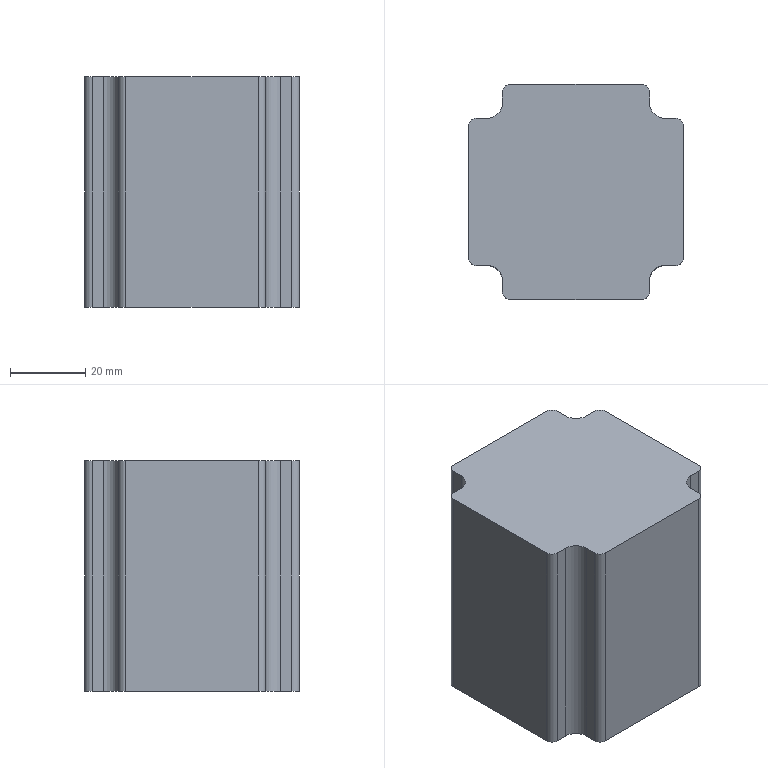Part | SolidWorks | features BaseBody 1 | 1 solid | 26 faces | box 57 x 57 x 61 mm | volume 178844 mm3 | plane 14 | cylinder 12 | commonest cylinder face diameters 4 x8 8 x4
STEP:
#1=CARTESIAN_POINT('',(19.5,26.5,0.));
#2=VERTEX_POINT('',#1);
#3=CARTESIAN_POINT('',(17.5,28.5,0.));
#4=VERTEX_POINT('',#3);
#5=CARTESIAN_POINT('',(17.5,26.5,0.));
#6=DIRECTION('',(0.,0.,1.));
#7=DIRECTION('',(-1.,0.,0.));
#8=AXIS2_PLACEMENT_3D('',#5,#6,#7);
#9=CIRCLE('',#8,2.);
#10=EDGE_CURVE('',#2,#4,#9,.T.);
#11=ORIENTED_EDGE('',*,*,#10,.T.);
#12=CARTESIAN_POINT('',(17.5,28.5,61.));
#13=VERTEX_POINT('',#12);
#14=CARTESIAN_POINT('',(17.5,28.5,61.));
#15=DIRECTION('',(0.,0.,-1.));
#16=VECTOR('',#15,1000.);
#17=LINE('',#14,#16);
#18=EDGE_CURVE('',#13,#4,#17,.T.);
#19=ORIENTED_EDGE('',*,*,#18,.F.);
#20=CARTESIAN_POINT('',(19.5,26.5,61.));
#21=VERTEX_POINT('',#20);
#22=CARTESIAN_POINT('',(17.5,26.5,61.));
#23=DIRECTION('',(0.,0.,1.));
#24=DIRECTION('',(-1.,0.,0.));
#25=AXIS2_PLACEMENT_3D('',#22,#23,#24);
#26=CIRCLE('',#25,2.);
#27=EDGE_CURVE('',#21,#13,#26,.T.);
#28=ORIENTED_EDGE('',*,*,#27,.F.);
#29=CARTESIAN_POINT('',(19.5,26.5,61.));
#30=DIRECTION('',(0.,0.,-1.));
#31=VECTOR('',#30,1000.);
#32=LINE('',#29,#31);
#33=EDGE_CURVE('',#21,#2,#32,.T.);
#34=ORIENTED_EDGE('',*,*,#33,.T.);
#35=EDGE_LOOP('',(#11,#19,#28,#34));
#36=FACE_OUTER_BOUND('',#35,.T.);
#37=CARTESIAN_POINT('',(17.5,26.5,61.));
#38=DIRECTION('',(0.,0.,-1.));
#39=DIRECTION('',(-1.,0.,0.));
#40=AXIS2_PLACEMENT_3D('',#37,#38,#39);
#41=CYLINDRICAL_SURFACE('',#40,2.);
#42=ADVANCED_FACE('',(#36),#41,.T.);
#43=CARTESIAN_POINT('',(-17.5,28.5,0.));
#44=VERTEX_POINT('',#43);
#45=CARTESIAN_POINT('',(-17.5,28.5,0.));
#46=DIRECTION('',(-1.,0.,0.));
#47=VECTOR('',#46,1000.);
#48=LINE('',#45,#47);
#49=EDGE_CURVE('',#4,#44,#48,.T.);
#50=ORIENTED_EDGE('',*,*,#49,.T.);
#51=CARTESIAN_POINT('',(-17.5,28.5,61.));
#52=VERTEX_POINT('',#51);
#53=CARTESIAN_POINT('',(-17.5,28.5,61.));
#54=DIRECTION('',(0.,0.,-1.));
#55=VECTOR('',#54,1000.);
#56=LINE('',#53,#55);
#57=EDGE_CURVE('',#52,#44,#56,.T.);
#58=ORIENTED_EDGE('',*,*,#57,.F.);
#59=CARTESIAN_POINT('',(-17.5,28.5,61.));
#60=DIRECTION('',(-1.,0.,0.));
#61=VECTOR('',#60,1000.);
#62=LINE('',#59,#61);
#63=EDGE_CURVE('',#13,#52,#62,.T.);
#64=ORIENTED_EDGE('',*,*,#63,.F.);
#65=ORIENTED_EDGE('',*,*,#18,.T.);
#66=EDGE_LOOP('',(#50,#58,#64,#65));
#67=FACE_OUTER_BOUND('',#66,.T.);
#68=CARTESIAN_POINT('',(-17.5,28.5,61.));
#69=DIRECTION('',(0.,-1.,0.));
#70=DIRECTION('',(0.,0.,-1.));
#71=AXIS2_PLACEMENT_3D('',#68,#69,#70);
#72=PLANE('',#71);
#73=ADVANCED_FACE('',(#67),#72,.F.);
#74=CARTESIAN_POINT('',(-19.5,26.5,0.));
#75=VERTEX_POINT('',#74);
#76=CARTESIAN_POINT('',(-17.5,26.5,0.));
#77=DIRECTION('',(0.,0.,1.));
#78=DIRECTION('',(-1.,0.,0.));
#79=AXIS2_PLACEMENT_3D('',#76,#77,#78);
#80=CIRCLE('',#79,2.);
#81=EDGE_CURVE('',#44,#75,#80,.T.);
#82=ORIENTED_EDGE('',*,*,#81,.T.);
#83=CARTESIAN_POINT('',(-19.5,26.5,61.));
#84=VERTEX_POINT('',#83);
#85=CARTESIAN_POINT('',(-19.5,26.5,61.));
#86=DIRECTION('',(0.,0.,-1.));
#87=VECTOR('',#86,1000.);
#88=LINE('',#85,#87);
#89=EDGE_CURVE('',#84,#75,#88,.T.);
#90=ORIENTED_EDGE('',*,*,#89,.F.);
#91=CARTESIAN_POINT('',(-17.5,26.5,61.));
#92=DIRECTION('',(0.,0.,1.));
#93=DIRECTION('',(-1.,0.,0.));
#94=AXIS2_PLACEMENT_3D('',#91,#92,#93);
#95=CIRCLE('',#94,2.);
#96=EDGE_CURVE('',#52,#84,#95,.T.);
#97=ORIENTED_EDGE('',*,*,#96,.F.);
#98=ORIENTED_EDGE('',*,*,#57,.T.);
#99=EDGE_LOOP('',(#82,#90,#97,#98));
#100=FACE_OUTER_BOUND('',#99,.T.);
#101=CARTESIAN_POINT('',(-17.5,26.5,61.));
#102=DIRECTION('',(0.,0.,-1.));
#103=DIRECTION('',(-1.,0.,0.));
#104=AXIS2_PLACEMENT_3D('',#101,#102,#103);
#105=CYLINDRICAL_SURFACE('',#104,2.);
#106=ADVANCED_FACE('',(#100),#105,.T.);
#107=CARTESIAN_POINT('',(-19.5,23.5,0.));
#108=VERTEX_POINT('',#107);
#109=CARTESIAN_POINT('',(-19.5,23.5,0.));
#110=DIRECTION('',(0.,-1.,0.));
#111=VECTOR('',#110,1000.);
#112=LINE('',#109,#111);
#113=EDGE_CURVE('',#75,#108,#112,.T.);
#114=ORIENTED_EDGE('',*,*,#113,.T.);
#115=CARTESIAN_POINT('',(-19.5,23.5,61.));
#116=VERTEX_POINT('',#115);
#117=CARTESIAN_POINT('',(-19.5,23.5,61.));
#118=DIRECTION('',(0.,0.,-1.));
#119=VECTOR('',#118,1000.);
#120=LINE('',#117,#119);
#121=EDGE_CURVE('',#116,#108,#120,.T.);
#122=ORIENTED_EDGE('',*,*,#121,.F.);
#123=CARTESIAN_POINT('',(-19.5,23.5,61.));
#124=DIRECTION('',(0.,-1.,0.));
#125=VECTOR('',#124,1000.);
#126=LINE('',#123,#125);
#127=EDGE_CURVE('',#84,#116,#126,.T.);
#128=ORIENTED_EDGE('',*,*,#127,.F.);
#129=ORIENTED_EDGE('',*,*,#89,.T.);
#130=EDGE_LOOP('',(#114,#122,#128,#129));
#131=FACE_OUTER_BOUND('',#130,.T.);
#132=CARTESIAN_POINT('',(-19.5,23.5,61.));
#133=DIRECTION('',(1.,0.,0.));
#134=DIRECTION('',(0.,1.,0.));
#135=AXIS2_PLACEMENT_3D('',#132,#133,#134);
#136=PLANE('',#135);
#137=ADVANCED_FACE('',(#131),#136,.F.);
#138=CARTESIAN_POINT('',(-23.5,19.5,0.));
#139=VERTEX_POINT('',#138);
#140=CARTESIAN_POINT('',(-23.5,23.5,0.));
#141=DIRECTION('',(0.,0.,-1.));
#142=DIRECTION('',(1.,0.,0.));
#143=AXIS2_PLACEMENT_3D('',#140,#141,#142);
#144=CIRCLE('',#143,4.);
#145=EDGE_CURVE('',#108,#139,#144,.T.);
#146=ORIENTED_EDGE('',*,*,#145,.T.);
#147=CARTESIAN_POINT('',(-23.5,19.5,61.));
#148=VERTEX_POINT('',#147);
#149=CARTESIAN_POINT('',(-23.5,19.5,61.));
#150=DIRECTION('',(0.,0.,-1.));
#151=VECTOR('',#150,1000.);
#152=LINE('',#149,#151);
#153=EDGE_CURVE('',#148,#139,#152,.T.);
#154=ORIENTED_EDGE('',*,*,#153,.F.);
#155=CARTESIAN_POINT('',(-23.5,23.5,61.));
#156=DIRECTION('',(0.,0.,-1.));
#157=DIRECTION('',(1.,0.,0.));
#158=AXIS2_PLACEMENT_3D('',#155,#156,#157);
#159=CIRCLE('',#158,4.);
#160=EDGE_CURVE('',#116,#148,#159,.T.);
#161=ORIENTED_EDGE('',*,*,#160,.F.);
#162=ORIENTED_EDGE('',*,*,#121,.T.);
#163=EDGE_LOOP('',(#146,#154,#161,#162));
#164=FACE_OUTER_BOUND('',#163,.T.);
#165=CARTESIAN_POINT('',(-23.5,23.5,61.));
#166=DIRECTION('',(0.,0.,-1.));
#167=DIRECTION('',(-1.,0.,0.));
#168=AXIS2_PLACEMENT_3D('',#165,#166,#167);
#169=CYLINDRICAL_SURFACE('',#168,4.);
#170=ADVANCED_FACE('',(#164),#169,.F.);
#171=CARTESIAN_POINT('',(-26.5,19.5,0.));
#172=VERTEX_POINT('',#171);
#173=CARTESIAN_POINT('',(-26.5,19.5,0.));
#174=DIRECTION('',(-1.,0.,0.));
#175=VECTOR('',#174,1000.);
#176=LINE('',#173,#175);
#177=EDGE_CURVE('',#139,#172,#176,.T.);
#178=ORIENTED_EDGE('',*,*,#177,.T.);
#179=CARTESIAN_POINT('',(-26.5,19.5,61.));
#180=VERTEX_POINT('',#179);
#181=CARTESIAN_POINT('',(-26.5,19.5,61.));
#182=DIRECTION('',(0.,0.,-1.));
#183=VECTOR('',#182,1000.);
#184=LINE('',#181,#183);
#185=EDGE_CURVE('',#180,#172,#184,.T.);
#186=ORIENTED_EDGE('',*,*,#185,.F.);
#187=CARTESIAN_POINT('',(-26.5,19.5,61.));
#188=DIRECTION('',(-1.,0.,0.));
#189=VECTOR('',#188,1000.);
#190=LINE('',#187,#189);
#191=EDGE_CURVE('',#148,#180,#190,.T.);
#192=ORIENTED_EDGE('',*,*,#191,.F.);
#193=ORIENTED_EDGE('',*,*,#153,.T.);
#194=EDGE_LOOP('',(#178,#186,#192,#193));
#195=FACE_OUTER_BOUND('',#194,.T.);
#196=CARTESIAN_POINT('',(-26.5,19.5,61.));
#197=DIRECTION('',(0.,-1.,0.));
#198=DIRECTION('',(0.,0.,-1.));
#199=AXIS2_PLACEMENT_3D('',#196,#197,#198);
#200=PLANE('',#199);
#201=ADVANCED_FACE('',(#195),#200,.F.);
#202=CARTESIAN_POINT('',(-28.5,17.5,0.));
#203=VERTEX_POINT('',#202);
#204=CARTESIAN_POINT('',(-26.5,17.5,0.));
#205=DIRECTION('',(0.,0.,1.));
#206=DIRECTION('',(-1.,0.,0.));
#207=AXIS2_PLACEMENT_3D('',#204,#205,#206);
#208=CIRCLE('',#207,2.);
#209=EDGE_CURVE('',#172,#203,#208,.T.);
#210=ORIENTED_EDGE('',*,*,#209,.T.);
#211=CARTESIAN_POINT('',(-28.5,17.5,61.));
#212=VERTEX_POINT('',#211);
#213=CARTESIAN_POINT('',(-28.5,17.5,61.));
#214=DIRECTION('',(0.,0.,-1.));
#215=VECTOR('',#214,1000.);
#216=LINE('',#213,#215);
#217=EDGE_CURVE('',#212,#203,#216,.T.);
#218=ORIENTED_EDGE('',*,*,#217,.F.);
#219=CARTESIAN_POINT('',(-26.5,17.5,61.));
#220=DIRECTION('',(0.,0.,1.));
#221=DIRECTION('',(-1.,0.,0.));
#222=AXIS2_PLACEMENT_3D('',#219,#220,#221);
#223=CIRCLE('',#222,2.);
#224=EDGE_CURVE('',#180,#212,#223,.T.);
#225=ORIENTED_EDGE('',*,*,#224,.F.);
#226=ORIENTED_EDGE('',*,*,#185,.T.);
#227=EDGE_LOOP('',(#210,#218,#225,#226));
#228=FACE_OUTER_BOUND('',#227,.T.);
#229=CARTESIAN_POINT('',(-26.5,17.5,61.));
#230=DIRECTION('',(0.,0.,-1.));
#231=DIRECTION('',(-1.,0.,0.));
#232=AXIS2_PLACEMENT_3D('',#229,#230,#231);
#233=CYLINDRICAL_SURFACE('',#232,2.);
#234=ADVANCED_FACE('',(#228),#233,.T.);
#235=CARTESIAN_POINT('',(-28.5,-17.5,0.));
#236=VERTEX_POINT('',#235);
#237=CARTESIAN_POINT('',(-28.5,-17.5,0.));
#238=DIRECTION('',(0.,-1.,0.));
#239=VECTOR('',#238,1000.);
#240=LINE('',#237,#239);
#241=EDGE_CURVE('',#203,#236,#240,.T.);
#242=ORIENTED_EDGE('',*,*,#241,.T.);
#243=CARTESIAN_POINT('',(-28.5,-17.5,61.));
#244=VERTEX_POINT('',#243);
#245=CARTESIAN_POINT('',(-28.5,-17.5,61.));
#246=DIRECTION('',(0.,0.,-1.));
#247=VECTOR('',#246,1000.);
#248=LINE('',#245,#247);
#249=EDGE_CURVE('',#244,#236,#248,.T.);
#250=ORIENTED_EDGE('',*,*,#249,.F.);
#251=CARTESIAN_POINT('',(-28.5,-17.5,61.));
#252=DIRECTION('',(0.,-1.,0.));
#253=VECTOR('',#252,1000.);
#254=LINE('',#251,#253);
#255=EDGE_CURVE('',#212,#244,#254,.T.);
#256=ORIENTED_EDGE('',*,*,#255,.F.);
#257=ORIENTED_EDGE('',*,*,#217,.T.);
#258=EDGE_LOOP('',(#242,#250,#256,#257));
#259=FACE_OUTER_BOUND('',#258,.T.);
#260=CARTESIAN_POINT('',(-28.5,-17.5,61.));
#261=DIRECTION('',(1.,0.,0.));
#262=DIRECTION('',(0.,1.,0.));
#263=AXIS2_PLACEMENT_3D('',#260,#261,#262);
#264=PLANE('',#263);
#265=ADVANCED_FACE('',(#259),#264,.F.);
#266=CARTESIAN_POINT('',(-26.5,-19.5,0.));
#267=VERTEX_POINT('',#266);
#268=CARTESIAN_POINT('',(-26.5,-17.5,0.));
#269=DIRECTION('',(0.,0.,1.));
#270=DIRECTION('',(-1.,0.,0.));
#271=AXIS2_PLACEMENT_3D('',#268,#269,#270);
#272=CIRCLE('',#271,2.);
#273=EDGE_CURVE('',#236,#267,#272,.T.);
#274=ORIENTED_EDGE('',*,*,#273,.T.);
#275=CARTESIAN_POINT('',(-26.5,-19.5,61.));
#276=VERTEX_POINT('',#275);
#277=CARTESIAN_POINT('',(-26.5,-19.5,61.));
#278=DIRECTION('',(0.,0.,-1.));
#279=VECTOR('',#278,1000.);
#280=LINE('',#277,#279);
#281=EDGE_CURVE('',#276,#267,#280,.T.);
#282=ORIENTED_EDGE('',*,*,#281,.F.);
#283=CARTESIAN_POINT('',(-26.5,-17.5,61.));
#284=DIRECTION('',(0.,0.,1.));
#285=DIRECTION('',(-1.,0.,0.));
#286=AXIS2_PLACEMENT_3D('',#283,#284,#285);
#287=CIRCLE('',#286,2.);
#288=EDGE_CURVE('',#244,#276,#287,.T.);
#289=ORIENTED_EDGE('',*,*,#288,.F.);
#290=ORIENTED_EDGE('',*,*,#249,.T.);
#291=EDGE_LOOP('',(#274,#282,#289,#290));
#292=FACE_OUTER_BOUND('',#291,.T.);
#293=CARTESIAN_POINT('',(-26.5,-17.5,61.));
#294=DIRECTION('',(0.,0.,-1.));
#295=DIRECTION('',(-1.,0.,0.));
#296=AXIS2_PLACEMENT_3D('',#293,#294,#295);
#297=CYLINDRICAL_SURFACE('',#296,2.);
#298=ADVANCED_FACE('',(#292),#297,.T.);
#299=CARTESIAN_POINT('',(-23.5,-19.5,0.));
#300=VERTEX_POINT('',#299);
#301=CARTESIAN_POINT('',(-23.5,-19.5,0.));
#302=DIRECTION('',(1.,0.,0.));
#303=VECTOR('',#302,1000.);
#304=LINE('',#301,#303);
#305=EDGE_CURVE('',#267,#300,#304,.T.);
#306=ORIENTED_EDGE('',*,*,#305,.T.);
#307=CARTESIAN_POINT('',(-23.5,-19.5,61.));
#308=VERTEX_POINT('',#307);
#309=CARTESIAN_POINT('',(-23.5,-19.5,61.));
#310=DIRECTION('',(0.,0.,-1.));
#311=VECTOR('',#310,1000.);
#312=LINE('',#309,#311);
#313=EDGE_CURVE('',#308,#300,#312,.T.);
#314=ORIENTED_EDGE('',*,*,#313,.F.);
#315=CARTESIAN_POINT('',(-23.5,-19.5,61.));
#316=DIRECTION('',(1.,0.,0.));
#317=VECTOR('',#316,1000.);
#318=LINE('',#315,#317);
#319=EDGE_CURVE('',#276,#308,#318,.T.);
#320=ORIENTED_EDGE('',*,*,#319,.F.);
#321=ORIENTED_EDGE('',*,*,#281,.T.);
#322=EDGE_LOOP('',(#306,#314,#320,#321));
#323=FACE_OUTER_BOUND('',#322,.T.);
#324=CARTESIAN_POINT('',(-23.5,-19.5,61.));
#325=DIRECTION('',(0.,1.,0.));
#326=DIRECTION('',(1.,0.,0.));
#327=AXIS2_PLACEMENT_3D('',#324,#325,#326);
#328=PLANE('',#327);
#329=ADVANCED_FACE('',(#323),#328,.F.);
#330=CARTESIAN_POINT('',(-19.5,-23.5,0.));
#331=VERTEX_POINT('',#330);
#332=CARTESIAN_POINT('',(-23.5,-23.5,0.));
#333=DIRECTION('',(0.,0.,-1.));
#334=DIRECTION('',(1.,0.,0.));
#335=AXIS2_PLACEMENT_3D('',#332,#333,#334);
#336=CIRCLE('',#335,4.);
#337=EDGE_CURVE('',#300,#331,#336,.T.);
#338=ORIENTED_EDGE('',*,*,#337,.T.);
#339=CARTESIAN_POINT('',(-19.5,-23.5,61.));
#340=VERTEX_POINT('',#339);
#341=CARTESIAN_POINT('',(-19.5,-23.5,61.));
#342=DIRECTION('',(0.,0.,-1.));
#343=VECTOR('',#342,1000.);
#344=LINE('',#341,#343);
#345=EDGE_CURVE('',#340,#331,#344,.T.);
#346=ORIENTED_EDGE('',*,*,#345,.F.);
#347=CARTESIAN_POINT('',(-23.5,-23.5,61.));
#348=DIRECTION('',(0.,0.,-1.));
#349=DIRECTION('',(1.,0.,0.));
#350=AXIS2_PLACEMENT_3D('',#347,#348,#349);
#351=CIRCLE('',#350,4.);
#352=EDGE_CURVE('',#308,#340,#351,.T.);
#353=ORIENTED_EDGE('',*,*,#352,.F.);
#354=ORIENTED_EDGE('',*,*,#313,.T.);
#355=EDGE_LOOP('',(#338,#346,#353,#354));
#356=FACE_OUTER_BOUND('',#355,.T.);
#357=CARTESIAN_POINT('',(-23.5,-23.5,61.));
#358=DIRECTION('',(0.,0.,-1.));
#359=DIRECTION('',(-1.,0.,0.));
#360=AXIS2_PLACEMENT_3D('',#357,#358,#359);
#361=CYLINDRICAL_SURFACE('',#360,4.);
#362=ADVANCED_FACE('',(#356),#361,.F.);
#363=CARTESIAN_POINT('',(-19.5,-26.5,0.));
#364=VERTEX_POINT('',#363);
#365=CARTESIAN_POINT('',(-19.5,-26.5,0.));
#366=DIRECTION('',(0.,-1.,0.));
#367=VECTOR('',#366,1000.);
#368=LINE('',#365,#367);
#369=EDGE_CURVE('',#331,#364,#368,.T.);
#370=ORIENTED_EDGE('',*,*,#369,.T.);
#371=CARTESIAN_POINT('',(-19.5,-26.5,61.));
#372=VERTEX_POINT('',#371);
#373=CARTESIAN_POINT('',(-19.5,-26.5,61.));
#374=DIRECTION('',(0.,0.,-1.));
#375=VECTOR('',#374,1000.);
#376=LINE('',#373,#375);
#377=EDGE_CURVE('',#372,#364,#376,.T.);
#378=ORIENTED_EDGE('',*,*,#377,.F.);
#379=CARTESIAN_POINT('',(-19.5,-26.5,61.));
#380=DIRECTION('',(0.,-1.,0.));
#381=VECTOR('',#380,1000.);
#382=LINE('',#379,#381);
#383=EDGE_CURVE('',#340,#372,#382,.T.);
#384=ORIENTED_EDGE('',*,*,#383,.F.);
#385=ORIENTED_EDGE('',*,*,#345,.T.);
#386=EDGE_LOOP('',(#370,#378,#384,#385));
#387=FACE_OUTER_BOUND('',#386,.T.);
#388=CARTESIAN_POINT('',(-19.5,-26.5,61.));
#389=DIRECTION('',(1.,0.,0.));
#390=DIRECTION('',(0.,1.,0.));
#391=AXIS2_PLACEMENT_3D('',#388,#389,#390);
#392=PLANE('',#391);
#393=ADVANCED_FACE('',(#387),#392,.F.);
#394=CARTESIAN_POINT('',(-17.5,-28.5,0.));
#395=VERTEX_POINT('',#394);
#396=CARTESIAN_POINT('',(-17.5,-26.5,0.));
#397=DIRECTION('',(0.,0.,1.));
#398=DIRECTION('',(-1.,0.,0.));
#399=AXIS2_PLACEMENT_3D('',#396,#397,#398);
#400=CIRCLE('',#399,2.);
#401=EDGE_CURVE('',#364,#395,#400,.T.);
#402=ORIENTED_EDGE('',*,*,#401,.T.);
#403=CARTESIAN_POINT('',(-17.5,-28.5,61.));
#404=VERTEX_POINT('',#403);
#405=CARTESIAN_POINT('',(-17.5,-28.5,61.));
#406=DIRECTION('',(0.,0.,-1.));
#407=VECTOR('',#406,1000.);
#408=LINE('',#405,#407);
#409=EDGE_CURVE('',#404,#395,#408,.T.);
#410=ORIENTED_EDGE('',*,*,#409,.F.);
#411=CARTESIAN_POINT('',(-17.5,-26.5,61.));
#412=DIRECTION('',(0.,0.,1.));
#413=DIRECTION('',(-1.,0.,0.));
#414=AXIS2_PLACEMENT_3D('',#411,#412,#413);
#415=CIRCLE('',#414,2.);
#416=EDGE_CURVE('',#372,#404,#415,.T.);
#417=ORIENTED_EDGE('',*,*,#416,.F.);
#418=ORIENTED_EDGE('',*,*,#377,.T.);
#419=EDGE_LOOP('',(#402,#410,#417,#418));
#420=FACE_OUTER_BOUND('',#419,.T.);
#421=CARTESIAN_POINT('',(-17.5,-26.5,61.));
#422=DIRECTION('',(0.,0.,-1.));
#423=DIRECTION('',(-1.,0.,0.));
#424=AXIS2_PLACEMENT_3D('',#421,#422,#423);
#425=CYLINDRICAL_SURFACE('',#424,2.);
#426=ADVANCED_FACE('',(#420),#425,.T.);
#427=CARTESIAN_POINT('',(17.5,-28.5,0.));
#428=VERTEX_POINT('',#427);
#429=CARTESIAN_POINT('',(17.5,-28.5,0.));
#430=DIRECTION('',(1.,0.,0.));
#431=VECTOR('',#430,1000.);
#432=LINE('',#429,#431);
#433=EDGE_CURVE('',#395,#428,#432,.T.);
#434=ORIENTED_EDGE('',*,*,#433,.T.);
#435=CARTESIAN_POINT('',(17.5,-28.5,61.));
#436=VERTEX_POINT('',#435);
#437=CARTESIAN_POINT('',(17.5,-28.5,61.));
#438=DIRECTION('',(0.,0.,-1.));
#439=VECTOR('',#438,1000.);
#440=LINE('',#437,#439);
#441=EDGE_CURVE('',#436,#428,#440,.T.);
#442=ORIENTED_EDGE('',*,*,#441,.F.);
#443=CARTESIAN_POINT('',(17.5,-28.5,61.));
#444=DIRECTION('',(1.,0.,0.));
#445=VECTOR('',#444,1000.);
#446=LINE('',#443,#445);
#447=EDGE_CURVE('',#404,#436,#446,.T.);
#448=ORIENTED_EDGE('',*,*,#447,.F.);
#449=ORIENTED_EDGE('',*,*,#409,.T.);
#450=EDGE_LOOP('',(#434,#442,#448,#449));
#451=FACE_OUTER_BOUND('',#450,.T.);
#452=CARTESIAN_POINT('',(17.5,-28.5,61.));
#453=DIRECTION('',(0.,1.,0.));
#454=DIRECTION('',(1.,0.,0.));
#455=AXIS2_PLACEMENT_3D('',#452,#453,#454);
#456=PLANE('',#455);
#457=ADVANCED_FACE('',(#451),#456,.F.);
#458=CARTESIAN_POINT('',(19.5,-26.5,0.));
#459=VERTEX_POINT('',#458);
#460=CARTESIAN_POINT('',(17.5,-26.5,0.));
#461=DIRECTION('',(0.,0.,1.));
#462=DIRECTION('',(-1.,0.,0.));
#463=AXIS2_PLACEMENT_3D('',#460,#461,#462);
#464=CIRCLE('',#463,2.);
#465=EDGE_CURVE('',#428,#459,#464,.T.);
#466=ORIENTED_EDGE('',*,*,#465,.T.);
#467=CARTESIAN_POINT('',(19.5,-26.5,61.));
#468=VERTEX_POINT('',#467);
#469=CARTESIAN_POINT('',(19.5,-26.5,61.));
#470=DIRECTION('',(0.,0.,-1.));
#471=VECTOR('',#470,1000.);
#472=LINE('',#469,#471);
#473=EDGE_CURVE('',#468,#459,#472,.T.);
#474=ORIENTED_EDGE('',*,*,#473,.F.);
#475=CARTESIAN_POINT('',(17.5,-26.5,61.));
#476=DIRECTION('',(0.,0.,1.));
#477=DIRECTION('',(-1.,0.,0.));
#478=AXIS2_PLACEMENT_3D('',#475,#476,#477);
#479=CIRCLE('',#478,2.);
#480=EDGE_CURVE('',#436,#468,#479,.T.);
#481=ORIENTED_EDGE('',*,*,#480,.F.);
#482=ORIENTED_EDGE('',*,*,#441,.T.);
#483=EDGE_LOOP('',(#466,#474,#481,#482));
#484=FACE_OUTER_BOUND('',#483,.T.);
#485=CARTESIAN_POINT('',(17.5,-26.5,61.));
#486=DIRECTION('',(0.,0.,-1.));
#487=DIRECTION('',(-1.,0.,0.));
#488=AXIS2_PLACEMENT_3D('',#485,#486,#487);
#489=CYLINDRICAL_SURFACE('',#488,2.);
#490=ADVANCED_FACE('',(#484),#489,.T.);
#491=CARTESIAN_POINT('',(19.5,-23.5,0.));
#492=VERTEX_POINT('',#491);
#493=CARTESIAN_POINT('',(19.5,-23.5,0.));
#494=DIRECTION('',(0.,1.,0.));
#495=VECTOR('',#494,1000.);
#496=LINE('',#493,#495);
#497=EDGE_CURVE('',#459,#492,#496,.T.);
#498=ORIENTED_EDGE('',*,*,#497,.T.);
#499=CARTESIAN_POINT('',(19.5,-23.5,61.));
#500=VERTEX_POINT('',#499);
#501=CARTESIAN_POINT('',(19.5,-23.5,61.));
#502=DIRECTION('',(0.,0.,-1.));
#503=VECTOR('',#502,1000.);
#504=LINE('',#501,#503);
#505=EDGE_CURVE('',#500,#492,#504,.T.);
#506=ORIENTED_EDGE('',*,*,#505,.F.);
#507=CARTESIAN_POINT('',(19.5,-23.5,61.));
#508=DIRECTION('',(0.,1.,0.));
#509=VECTOR('',#508,1000.);
#510=LINE('',#507,#509);
#511=EDGE_CURVE('',#468,#500,#510,.T.);
#512=ORIENTED_EDGE('',*,*,#511,.F.);
#513=ORIENTED_EDGE('',*,*,#473,.T.);
#514=EDGE_LOOP('',(#498,#506,#512,#513));
#515=FACE_OUTER_BOUND('',#514,.T.);
#516=CARTESIAN_POINT('',(19.5,-23.5,61.));
#517=DIRECTION('',(-1.,0.,0.));
#518=DIRECTION('',(0.,0.,1.));
#519=AXIS2_PLACEMENT_3D('',#516,#517,#518);
#520=PLANE('',#519);
#521=ADVANCED_FACE('',(#515),#520,.F.);
#522=CARTESIAN_POINT('',(23.5,-19.5,0.));
#523=VERTEX_POINT('',#522);
#524=CARTESIAN_POINT('',(23.5,-23.5,0.));
#525=DIRECTION('',(0.,0.,-1.));
#526=DIRECTION('',(-1.,0.,0.));
#527=AXIS2_PLACEMENT_3D('',#524,#525,#526);
#528=CIRCLE('',#527,4.);
#529=EDGE_CURVE('',#492,#523,#528,.T.);
#530=ORIENTED_EDGE('',*,*,#529,.T.);
#531=CARTESIAN_POINT('',(23.5,-19.5,61.));
#532=VERTEX_POINT('',#531);
#533=CARTESIAN_POINT('',(23.5,-19.5,61.));
#534=DIRECTION('',(0.,0.,-1.));
#535=VECTOR('',#534,1000.);
#536=LINE('',#533,#535);
#537=EDGE_CURVE('',#532,#523,#536,.T.);
#538=ORIENTED_EDGE('',*,*,#537,.F.);
#539=CARTESIAN_POINT('',(23.5,-23.5,61.));
#540=DIRECTION('',(0.,0.,-1.));
#541=DIRECTION('',(-1.,0.,0.));
#542=AXIS2_PLACEMENT_3D('',#539,#540,#541);
#543=CIRCLE('',#542,4.);
#544=EDGE_CURVE('',#500,#532,#543,.T.);
#545=ORIENTED_EDGE('',*,*,#544,.F.);
#546=ORIENTED_EDGE('',*,*,#505,.T.);
#547=EDGE_LOOP('',(#530,#538,#545,#546));
#548=FACE_OUTER_BOUND('',#547,.T.);
#549=CARTESIAN_POINT('',(23.5,-23.5,61.));
#550=DIRECTION('',(0.,0.,-1.));
#551=DIRECTION('',(-1.,0.,0.));
#552=AXIS2_PLACEMENT_3D('',#549,#550,#551);
#553=CYLINDRICAL_SURFACE('',#552,4.);
#554=ADVANCED_FACE('',(#548),#553,.F.);
#555=CARTESIAN_POINT('',(26.5,-19.5,0.));
#556=VERTEX_POINT('',#555);
#557=CARTESIAN_POINT('',(26.5,-19.5,0.));
#558=DIRECTION('',(1.,0.,0.));
#559=VECTOR('',#558,1000.);
#560=LINE('',#557,#559);
#561=EDGE_CURVE('',#523,#556,#560,.T.);
#562=ORIENTED_EDGE('',*,*,#561,.T.);
#563=CARTESIAN_POINT('',(26.5,-19.5,61.));
#564=VERTEX_POINT('',#563);
#565=CARTESIAN_POINT('',(26.5,-19.5,61.));
#566=DIRECTION('',(0.,0.,-1.));
#567=VECTOR('',#566,1000.);
#568=LINE('',#565,#567);
#569=EDGE_CURVE('',#564,#556,#568,.T.);
#570=ORIENTED_EDGE('',*,*,#569,.F.);
#571=CARTESIAN_POINT('',(26.5,-19.5,61.));
#572=DIRECTION('',(1.,0.,0.));
#573=VECTOR('',#572,1000.);
#574=LINE('',#571,#573);
#575=EDGE_CURVE('',#532,#564,#574,.T.);
#576=ORIENTED_EDGE('',*,*,#575,.F.);
#577=ORIENTED_EDGE('',*,*,#537,.T.);
#578=EDGE_LOOP('',(#562,#570,#576,#577));
#579=FACE_OUTER_BOUND('',#578,.T.);
#580=CARTESIAN_POINT('',(26.5,-19.5,61.));
#581=DIRECTION('',(0.,1.,0.));
#582=DIRECTION('',(1.,0.,0.));
#583=AXIS2_PLACEMENT_3D('',#580,#581,#582);
#584=PLANE('',#583);
#585=ADVANCED_FACE('',(#579),#584,.F.);
#586=CARTESIAN_POINT('',(28.5,-17.5,0.));
#587=VERTEX_POINT('',#586);
#588=CARTESIAN_POINT('',(26.5,-17.5,0.));
#589=DIRECTION('',(0.,0.,1.));
#590=DIRECTION('',(-1.,0.,0.));
#591=AXIS2_PLACEMENT_3D('',#588,#589,#590);
#592=CIRCLE('',#591,2.);
#593=EDGE_CURVE('',#556,#587,#592,.T.);
#594=ORIENTED_EDGE('',*,*,#593,.T.);
#595=CARTESIAN_POINT('',(28.5,-17.5,61.));
#596=VERTEX_POINT('',#595);
#597=CARTESIAN_POINT('',(28.5,-17.5,61.));
#598=DIRECTION('',(0.,0.,-1.));
#599=VECTOR('',#598,1000.);
#600=LINE('',#597,#599);
#601=EDGE_CURVE('',#596,#587,#600,.T.);
#602=ORIENTED_EDGE('',*,*,#601,.F.);
#603=CARTESIAN_POINT('',(26.5,-17.5,61.));
#604=DIRECTION('',(0.,0.,1.));
#605=DIRECTION('',(-1.,0.,0.));
#606=AXIS2_PLACEMENT_3D('',#603,#604,#605);
#607=CIRCLE('',#606,2.);
#608=EDGE_CURVE('',#564,#596,#607,.T.);
#609=ORIENTED_EDGE('',*,*,#608,.F.);
#610=ORIENTED_EDGE('',*,*,#569,.T.);
#611=EDGE_LOOP('',(#594,#602,#609,#610));
#612=FACE_OUTER_BOUND('',#611,.T.);
#613=CARTESIAN_POINT('',(26.5,-17.5,61.));
#614=DIRECTION('',(0.,0.,-1.));
#615=DIRECTION('',(-1.,0.,0.));
#616=AXIS2_PLACEMENT_3D('',#613,#614,#615);
#617=CYLINDRICAL_SURFACE('',#616,2.);
#618=ADVANCED_FACE('',(#612),#617,.T.);
#619=CARTESIAN_POINT('',(28.5,17.5,0.));
#620=VERTEX_POINT('',#619);
#621=CARTESIAN_POINT('',(28.5,17.5,0.));
#622=DIRECTION('',(0.,1.,0.));
#623=VECTOR('',#622,1000.);
#624=LINE('',#621,#623);
#625=EDGE_CURVE('',#587,#620,#624,.T.);
#626=ORIENTED_EDGE('',*,*,#625,.T.);
#627=CARTESIAN_POINT('',(28.5,17.5,61.));
#628=VERTEX_POINT('',#627);
#629=CARTESIAN_POINT('',(28.5,17.5,61.));
#630=DIRECTION('',(0.,0.,-1.));
#631=VECTOR('',#630,1000.);
#632=LINE('',#629,#631);
#633=EDGE_CURVE('',#628,#620,#632,.T.);
#634=ORIENTED_EDGE('',*,*,#633,.F.);
#635=CARTESIAN_POINT('',(28.5,17.5,61.));
#636=DIRECTION('',(0.,1.,0.));
#637=VECTOR('',#636,1000.);
#638=LINE('',#635,#637);
#639=EDGE_CURVE('',#596,#628,#638,.T.);
#640=ORIENTED_EDGE('',*,*,#639,.F.);
#641=ORIENTED_EDGE('',*,*,#601,.T.);
#642=EDGE_LOOP('',(#626,#634,#640,#641));
#643=FACE_OUTER_BOUND('',#642,.T.);
#644=CARTESIAN_POINT('',(28.5,17.5,61.));
#645=DIRECTION('',(-1.,0.,0.));
#646=DIRECTION('',(0.,1.,0.));
#647=AXIS2_PLACEMENT_3D('',#644,#645,#646);
#648=PLANE('',#647);
#649=ADVANCED_FACE('',(#643),#648,.F.);
#650=CARTESIAN_POINT('',(26.5,19.5,0.));
#651=VERTEX_POINT('',#650);
#652=CARTESIAN_POINT('',(26.5,17.5,0.));
#653=DIRECTION('',(0.,0.,1.));
#654=DIRECTION('',(-1.,0.,0.));
#655=AXIS2_PLACEMENT_3D('',#652,#653,#654);
#656=CIRCLE('',#655,2.);
#657=EDGE_CURVE('',#620,#651,#656,.T.);
#658=ORIENTED_EDGE('',*,*,#657,.T.);
#659=CARTESIAN_POINT('',(26.5,19.5,61.));
#660=VERTEX_POINT('',#659);
#661=CARTESIAN_POINT('',(26.5,19.5,61.));
#662=DIRECTION('',(0.,0.,-1.));
#663=VECTOR('',#662,1000.);
#664=LINE('',#661,#663);
#665=EDGE_CURVE('',#660,#651,#664,.T.);
#666=ORIENTED_EDGE('',*,*,#665,.F.);
#667=CARTESIAN_POINT('',(26.5,17.5,61.));
#668=DIRECTION('',(0.,0.,1.));
#669=DIRECTION('',(-1.,0.,0.));
#670=AXIS2_PLACEMENT_3D('',#667,#668,#669);
#671=CIRCLE('',#670,2.);
#672=EDGE_CURVE('',#628,#660,#671,.T.);
#673=ORIENTED_EDGE('',*,*,#672,.F.);
#674=ORIENTED_EDGE('',*,*,#633,.T.);
#675=EDGE_LOOP('',(#658,#666,#673,#674));
#676=FACE_OUTER_BOUND('',#675,.T.);
#677=CARTESIAN_POINT('',(26.5,17.5,61.));
#678=DIRECTION('',(0.,0.,-1.));
#679=DIRECTION('',(-1.,0.,0.));
#680=AXIS2_PLACEMENT_3D('',#677,#678,#679);
#681=CYLINDRICAL_SURFACE('',#680,2.);
#682=ADVANCED_FACE('',(#676),#681,.T.);
#683=CARTESIAN_POINT('',(23.5,19.5,0.));
#684=VERTEX_POINT('',#683);
#685=CARTESIAN_POINT('',(23.5,19.5,0.));
#686=DIRECTION('',(-1.,0.,0.));
#687=VECTOR('',#686,1000.);
#688=LINE('',#685,#687);
#689=EDGE_CURVE('',#651,#684,#688,.T.);
#690=ORIENTED_EDGE('',*,*,#689,.T.);
#691=CARTESIAN_POINT('',(23.5,19.5,61.));
#692=VERTEX_POINT('',#691);
#693=CARTESIAN_POINT('',(23.5,19.5,61.));
#694=DIRECTION('',(0.,0.,-1.));
#695=VECTOR('',#694,1000.);
#696=LINE('',#693,#695);
#697=EDGE_CURVE('',#692,#684,#696,.T.);
#698=ORIENTED_EDGE('',*,*,#697,.F.);
#699=CARTESIAN_POINT('',(23.5,19.5,61.));
#700=DIRECTION('',(-1.,0.,0.));
#701=VECTOR('',#700,1000.);
#702=LINE('',#699,#701);
#703=EDGE_CURVE('',#660,#692,#702,.T.);
#704=ORIENTED_EDGE('',*,*,#703,.F.);
#705=ORIENTED_EDGE('',*,*,#665,.T.);
#706=EDGE_LOOP('',(#690,#698,#704,#705));
#707=FACE_OUTER_BOUND('',#706,.T.);
#708=CARTESIAN_POINT('',(23.5,19.5,61.));
#709=DIRECTION('',(0.,-1.,0.));
#710=DIRECTION('',(0.,0.,-1.));
#711=AXIS2_PLACEMENT_3D('',#708,#709,#710);
#712=PLANE('',#711);
#713=ADVANCED_FACE('',(#707),#712,.F.);
#714=CARTESIAN_POINT('',(19.5,23.5,0.));
#715=VERTEX_POINT('',#714);
#716=CARTESIAN_POINT('',(23.5,23.5,0.));
#717=DIRECTION('',(0.,0.,-1.));
#718=DIRECTION('',(1.,0.,0.));
#719=AXIS2_PLACEMENT_3D('',#716,#717,#718);
#720=CIRCLE('',#719,4.);
#721=EDGE_CURVE('',#684,#715,#720,.T.);
#722=ORIENTED_EDGE('',*,*,#721,.T.);
#723=CARTESIAN_POINT('',(19.5,23.5,61.));
#724=VERTEX_POINT('',#723);
#725=CARTESIAN_POINT('',(19.5,23.5,61.));
#726=DIRECTION('',(0.,0.,-1.));
#727=VECTOR('',#726,1000.);
#728=LINE('',#725,#727);
#729=EDGE_CURVE('',#724,#715,#728,.T.);
#730=ORIENTED_EDGE('',*,*,#729,.F.);
#731=CARTESIAN_POINT('',(23.5,23.5,61.));
#732=DIRECTION('',(0.,0.,-1.));
#733=DIRECTION('',(1.,0.,0.));
#734=AXIS2_PLACEMENT_3D('',#731,#732,#733);
#735=CIRCLE('',#734,4.);
#736=EDGE_CURVE('',#692,#724,#735,.T.);
#737=ORIENTED_EDGE('',*,*,#736,.F.);
#738=ORIENTED_EDGE('',*,*,#697,.T.);
#739=EDGE_LOOP('',(#722,#730,#737,#738));
#740=FACE_OUTER_BOUND('',#739,.T.);
#741=CARTESIAN_POINT('',(23.5,23.5,61.));
#742=DIRECTION('',(0.,0.,-1.));
#743=DIRECTION('',(-1.,0.,0.));
#744=AXIS2_PLACEMENT_3D('',#741,#742,#743);
#745=CYLINDRICAL_SURFACE('',#744,4.);
#746=ADVANCED_FACE('',(#740),#745,.F.);
#747=CARTESIAN_POINT('',(19.5,26.5,0.));
#748=DIRECTION('',(0.,1.,0.));
#749=VECTOR('',#748,1000.);
#750=LINE('',#747,#749);
#751=EDGE_CURVE('',#715,#2,#750,.T.);
#752=ORIENTED_EDGE('',*,*,#751,.T.);
#753=ORIENTED_EDGE('',*,*,#33,.F.);
#754=CARTESIAN_POINT('',(19.5,26.5,61.));
#755=DIRECTION('',(0.,1.,0.));
#756=VECTOR('',#755,1000.);
#757=LINE('',#754,#756);
#758=EDGE_CURVE('',#724,#21,#757,.T.);
#759=ORIENTED_EDGE('',*,*,#758,.F.);
#760=ORIENTED_EDGE('',*,*,#729,.T.);
#761=EDGE_LOOP('',(#752,#753,#759,#760));
#762=FACE_OUTER_BOUND('',#761,.T.);
#763=CARTESIAN_POINT('',(19.5,26.5,61.));
#764=DIRECTION('',(-1.,0.,0.));
#765=DIRECTION('',(0.,0.,1.));
#766=AXIS2_PLACEMENT_3D('',#763,#764,#765);
#767=PLANE('',#766);
#768=ADVANCED_FACE('',(#762),#767,.F.);
#769=ORIENTED_EDGE('',*,*,#27,.T.);
#770=ORIENTED_EDGE('',*,*,#63,.T.);
#771=ORIENTED_EDGE('',*,*,#96,.T.);
#772=ORIENTED_EDGE('',*,*,#127,.T.);
#773=ORIENTED_EDGE('',*,*,#160,.T.);
#774=ORIENTED_EDGE('',*,*,#191,.T.);
#775=ORIENTED_EDGE('',*,*,#224,.T.);
#776=ORIENTED_EDGE('',*,*,#255,.T.);
#777=ORIENTED_EDGE('',*,*,#288,.T.);
#778=ORIENTED_EDGE('',*,*,#319,.T.);
#779=ORIENTED_EDGE('',*,*,#352,.T.);
#780=ORIENTED_EDGE('',*,*,#383,.T.);
#781=ORIENTED_EDGE('',*,*,#416,.T.);
#782=ORIENTED_EDGE('',*,*,#447,.T.);
#783=ORIENTED_EDGE('',*,*,#480,.T.);
#784=ORIENTED_EDGE('',*,*,#511,.T.);
#785=ORIENTED_EDGE('',*,*,#544,.T.);
#786=ORIENTED_EDGE('',*,*,#575,.T.);
#787=ORIENTED_EDGE('',*,*,#608,.T.);
#788=ORIENTED_EDGE('',*,*,#639,.T.);
#789=ORIENTED_EDGE('',*,*,#672,.T.);
#790=ORIENTED_EDGE('',*,*,#703,.T.);
#791=ORIENTED_EDGE('',*,*,#736,.T.);
#792=ORIENTED_EDGE('',*,*,#758,.T.);
#793=EDGE_LOOP('',(#769,#770,#771,#772,#773,#774,#775,#776,#777,#778,#779,#780,#781,#782,#783,#784,#785,#786,#787,#788,#789,#790,#791,#792));
#794=FACE_OUTER_BOUND('',#793,.T.);
#795=CARTESIAN_POINT('',(17.5,26.5,61.));
#796=DIRECTION('',(0.,0.,-1.));
#797=DIRECTION('',(0.,-1.,0.));
#798=AXIS2_PLACEMENT_3D('',#795,#796,#797);
#799=PLANE('',#798);
#800=ADVANCED_FACE('',(#794),#799,.F.);
#801=ORIENTED_EDGE('',*,*,#10,.F.);
#802=ORIENTED_EDGE('',*,*,#751,.F.);
#803=ORIENTED_EDGE('',*,*,#721,.F.);
#804=ORIENTED_EDGE('',*,*,#689,.F.);
#805=ORIENTED_EDGE('',*,*,#657,.F.);
#806=ORIENTED_EDGE('',*,*,#625,.F.);
#807=ORIENTED_EDGE('',*,*,#593,.F.);
#808=ORIENTED_EDGE('',*,*,#561,.F.);
#809=ORIENTED_EDGE('',*,*,#529,.F.);
#810=ORIENTED_EDGE('',*,*,#497,.F.);
#811=ORIENTED_EDGE('',*,*,#465,.F.);
#812=ORIENTED_EDGE('',*,*,#433,.F.);
#813=ORIENTED_EDGE('',*,*,#401,.F.);
#814=ORIENTED_EDGE('',*,*,#369,.F.);
#815=ORIENTED_EDGE('',*,*,#337,.F.);
#816=ORIENTED_EDGE('',*,*,#305,.F.);
#817=ORIENTED_EDGE('',*,*,#273,.F.);
#818=ORIENTED_EDGE('',*,*,#241,.F.);
#819=ORIENTED_EDGE('',*,*,#209,.F.);
#820=ORIENTED_EDGE('',*,*,#177,.F.);
#821=ORIENTED_EDGE('',*,*,#145,.F.);
#822=ORIENTED_EDGE('',*,*,#113,.F.);
#823=ORIENTED_EDGE('',*,*,#81,.F.);
#824=ORIENTED_EDGE('',*,*,#49,.F.);
#825=EDGE_LOOP('',(#801,#802,#803,#804,#805,#806,#807,#808,#809,#810,#811,#812,#813,#814,#815,#816,#817,#818,#819,#820,#821,#822,#823,#824));
#826=FACE_OUTER_BOUND('',#825,.T.);
#827=CARTESIAN_POINT('',(17.5,26.5,0.));
#828=DIRECTION('',(0.,0.,-1.));
#829=DIRECTION('',(0.,-1.,0.));
#830=AXIS2_PLACEMENT_3D('',#827,#828,#829);
#831=PLANE('',#830);
#832=ADVANCED_FACE('',(#826),#831,.T.);
#833=CLOSED_SHELL('',(#42,#73,#106,#137,#170,#201,#234,#265,#298,#329,#362,#393,#426,#457,#490,#521,#554,#585,#618,#649,#682,#713,#746,#768,#800,#832));
#834=MANIFOLD_SOLID_BREP('',#833);
#835=CARTESIAN_POINT('',(0.,0.,0.));
#836=DIRECTION('',(0.,0.,1.));
#837=DIRECTION('',(1.,0.,0.));
#838=AXIS2_PLACEMENT_3D('',#835,#836,#837);
#839=(LENGTH_UNIT()NAMED_UNIT(*)SI_UNIT(.MILLI.,.METRE.));
#840=UNCERTAINTY_MEASURE_WITH_UNIT(LENGTH_MEASURE(0.00001),#839,'','');
#841=(NAMED_UNIT(*)PLANE_ANGLE_UNIT()SI_UNIT($,.RADIAN.));
#842=(NAMED_UNIT(*)SI_UNIT($,.STERADIAN.)SOLID_ANGLE_UNIT());
#843=(GEOMETRIC_REPRESENTATION_CONTEXT(3)GLOBAL_UNCERTAINTY_ASSIGNED_CONTEXT((#840))GLOBAL_UNIT_ASSIGNED_CONTEXT((#839,#841,#842))REPRESENTATION_CONTEXT('',''));
#844=ADVANCED_BREP_SHAPE_REPRESENTATION('',(#834,#838),#843);